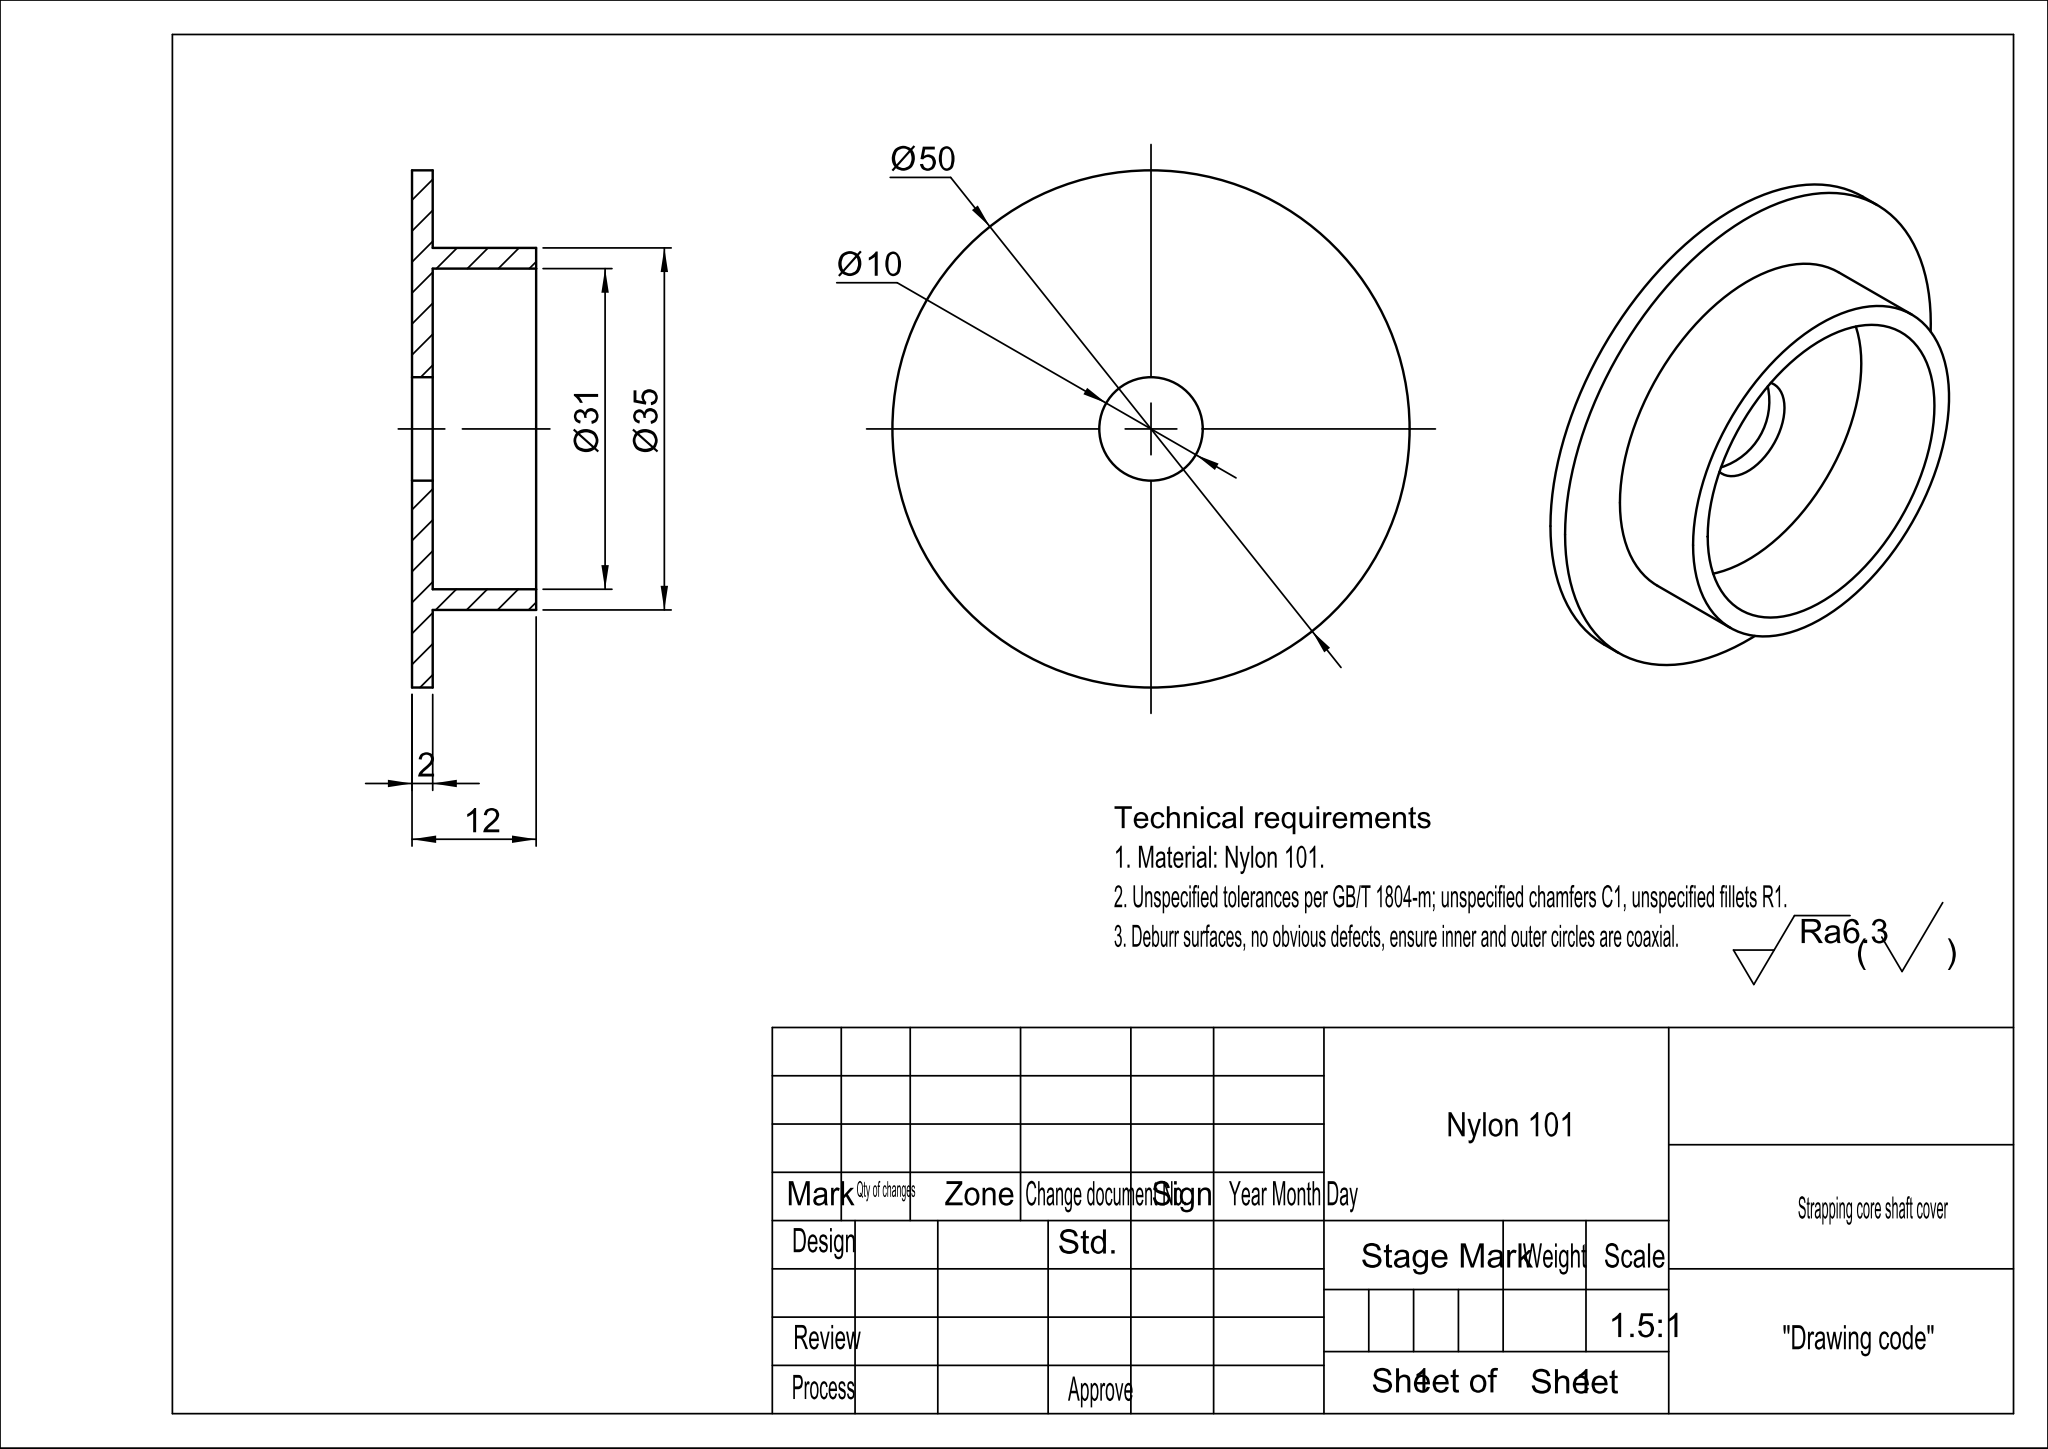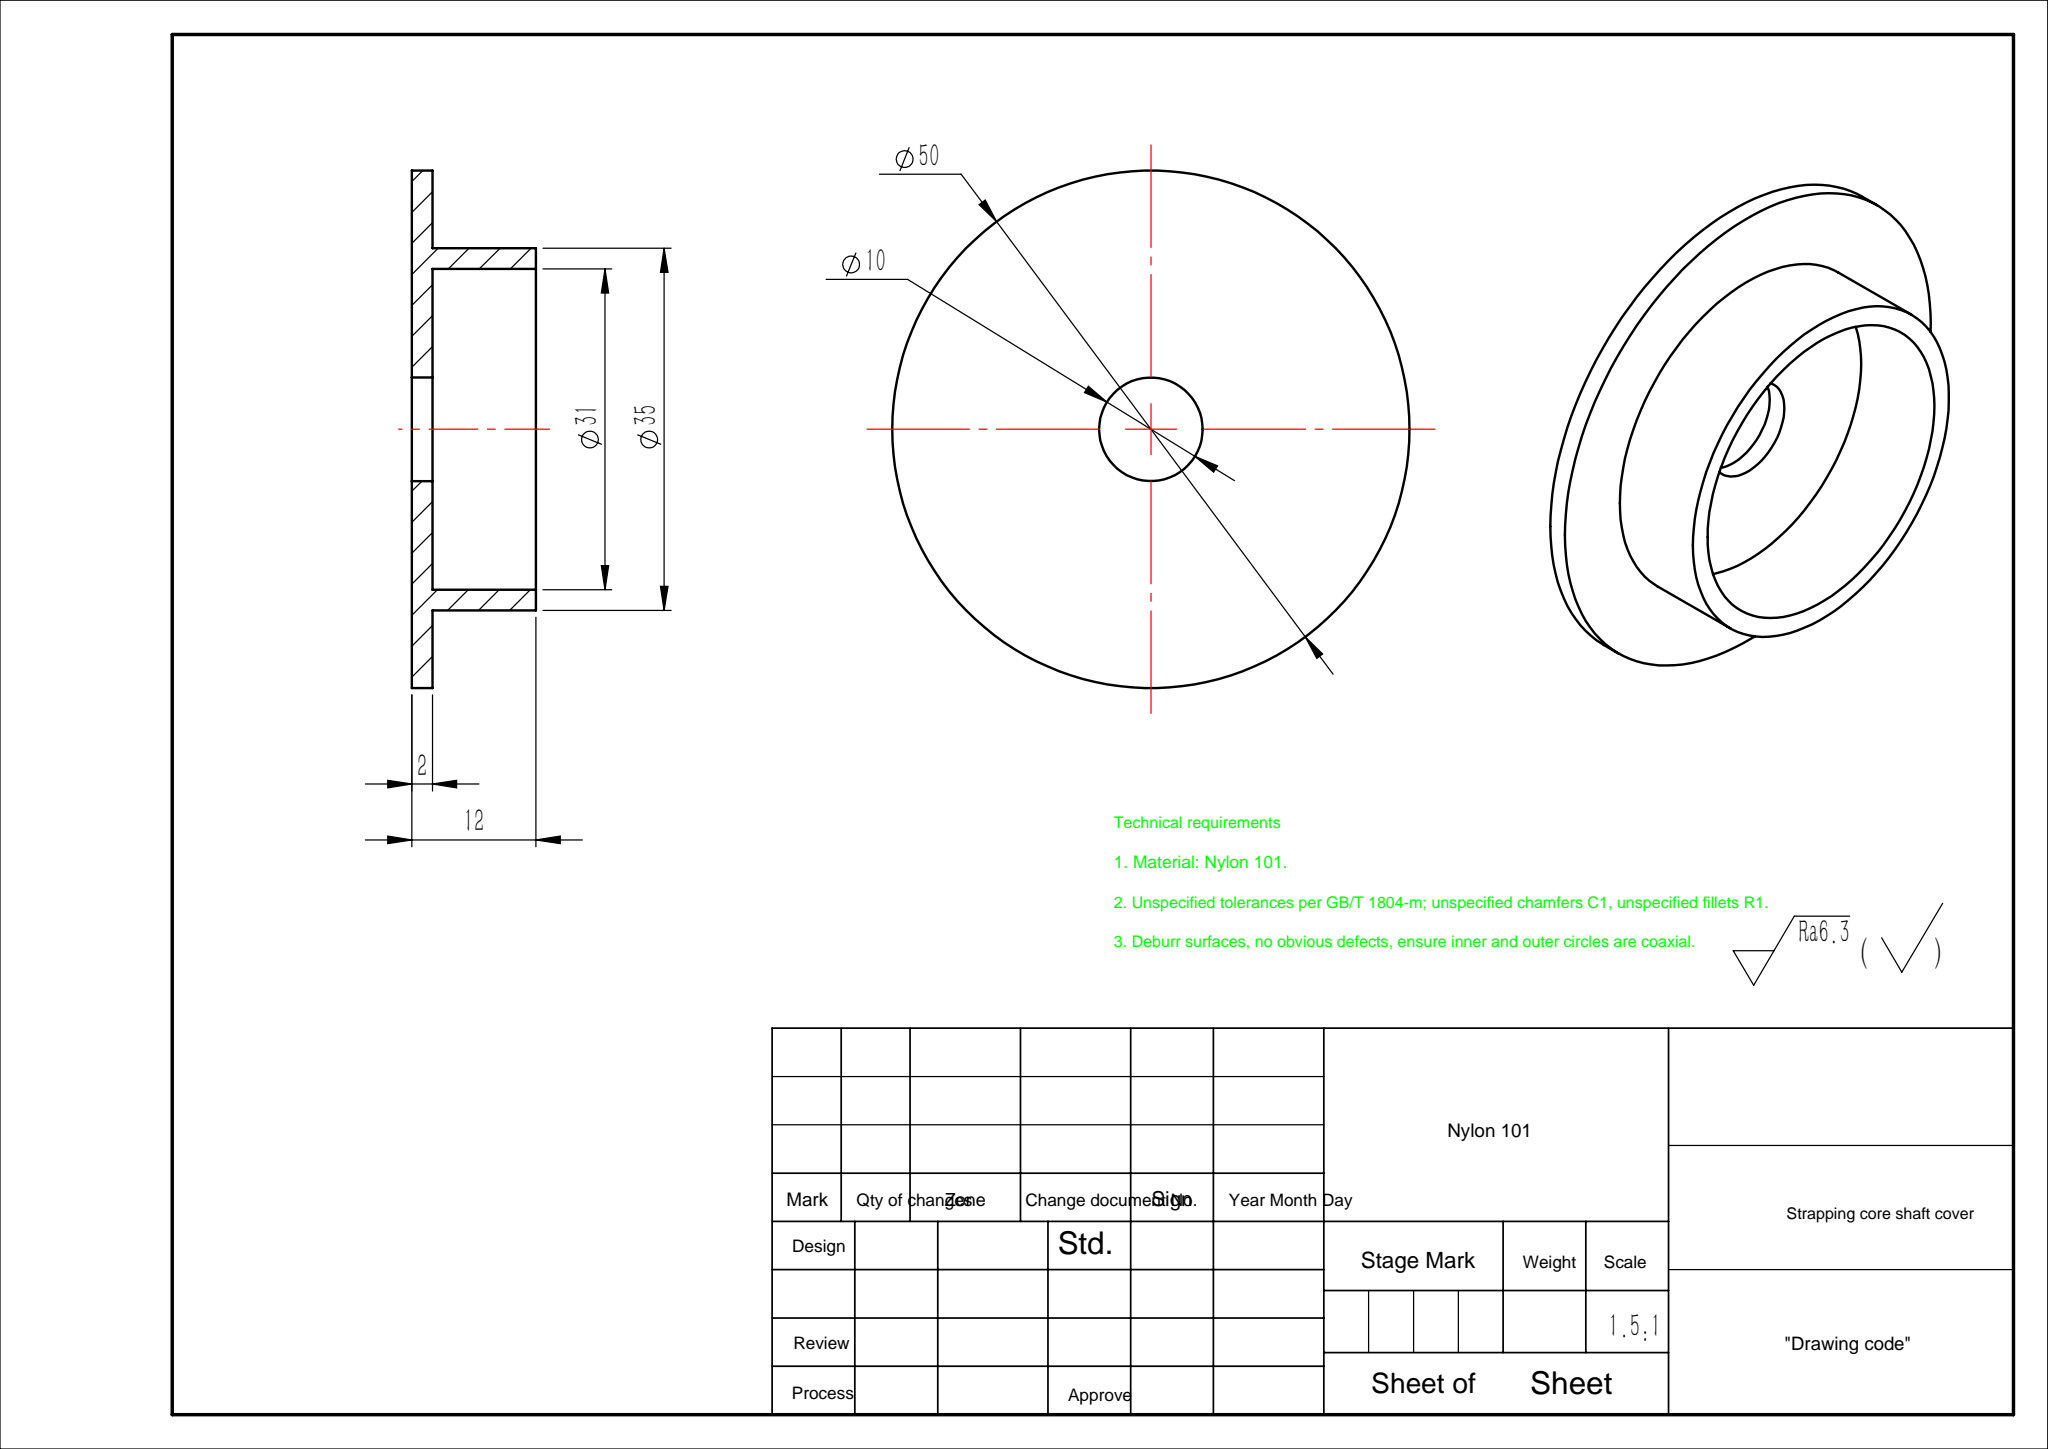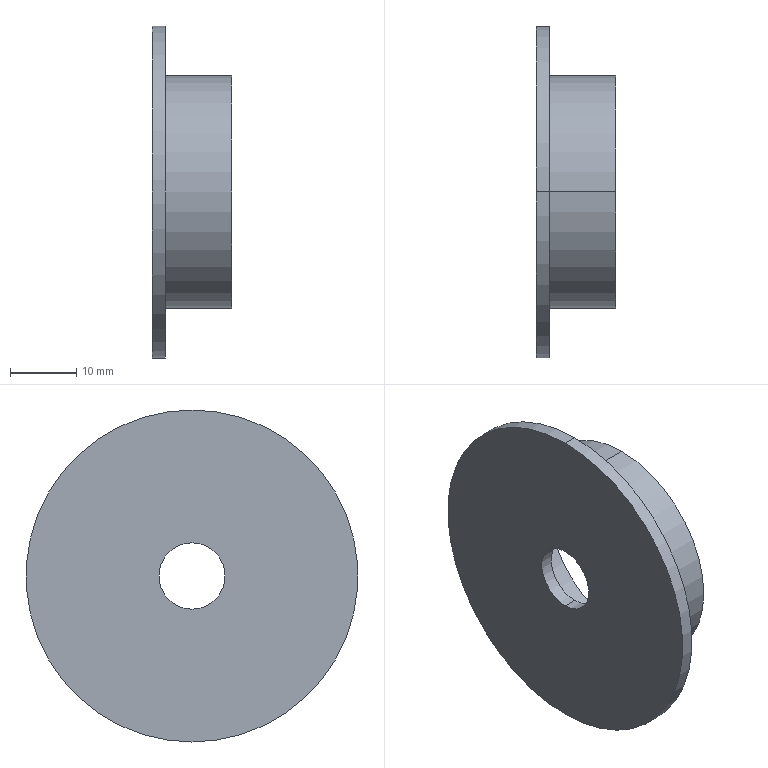Part | SolidWorks | features Revolution 1 | 1 solid | 12 faces | box 12 x 50 x 50 mm | volume 5843 mm3 | cylinder 8 | plane 4 | commonest cylinder face diameters 10 x2 31 x2 35 x2 50 x2
STEP:
#1=CARTESIAN_POINT('',(2.,0.,-5.));
#2=VERTEX_POINT('',#1);
#3=CARTESIAN_POINT('',(2.,0.,5.));
#4=VERTEX_POINT('',#3);
#5=CARTESIAN_POINT('',(2.,0.,0.));
#6=DIRECTION('',(-1.,0.,0.));
#7=DIRECTION('',(0.,0.,1.));
#8=AXIS2_PLACEMENT_3D('',#5,#6,#7);
#9=CIRCLE('',#8,5.);
#10=EDGE_CURVE('',#2,#4,#9,.T.);
#11=ORIENTED_EDGE('',*,*,#10,.F.);
#12=CARTESIAN_POINT('',(0.,0.,-5.));
#13=VERTEX_POINT('',#12);
#14=CARTESIAN_POINT('',(0.,0.,-5.));
#15=DIRECTION('',(-1.,0.,0.));
#16=VECTOR('',#15,1000.);
#17=LINE('',#14,#16);
#18=EDGE_CURVE('',#2,#13,#17,.T.);
#19=ORIENTED_EDGE('',*,*,#18,.T.);
#20=CARTESIAN_POINT('',(0.,0.,5.));
#21=VERTEX_POINT('',#20);
#22=CARTESIAN_POINT('',(0.,0.,0.));
#23=DIRECTION('',(-1.,0.,0.));
#24=DIRECTION('',(0.,0.,1.));
#25=AXIS2_PLACEMENT_3D('',#22,#23,#24);
#26=CIRCLE('',#25,5.);
#27=EDGE_CURVE('',#13,#21,#26,.T.);
#28=ORIENTED_EDGE('',*,*,#27,.T.);
#29=CARTESIAN_POINT('',(0.,0.,5.));
#30=DIRECTION('',(-1.,0.,0.));
#31=VECTOR('',#30,1000.);
#32=LINE('',#29,#31);
#33=EDGE_CURVE('',#4,#21,#32,.T.);
#34=ORIENTED_EDGE('',*,*,#33,.F.);
#35=EDGE_LOOP('',(#11,#19,#28,#34));
#36=FACE_OUTER_BOUND('',#35,.T.);
#37=CARTESIAN_POINT('',(0.,0.,0.));
#38=DIRECTION('',(-1.,0.,0.));
#39=DIRECTION('',(0.,0.,1.));
#40=AXIS2_PLACEMENT_3D('',#37,#38,#39);
#41=CYLINDRICAL_SURFACE('',#40,5.);
#42=ADVANCED_FACE('',(#36),#41,.F.);
#43=CARTESIAN_POINT('',(12.,0.,-15.5));
#44=VERTEX_POINT('',#43);
#45=CARTESIAN_POINT('',(12.,0.,15.5));
#46=VERTEX_POINT('',#45);
#47=CARTESIAN_POINT('',(12.,0.,0.));
#48=DIRECTION('',(-1.,0.,0.));
#49=DIRECTION('',(0.,0.,1.));
#50=AXIS2_PLACEMENT_3D('',#47,#48,#49);
#51=CIRCLE('',#50,15.5);
#52=EDGE_CURVE('',#44,#46,#51,.T.);
#53=ORIENTED_EDGE('',*,*,#52,.F.);
#54=CARTESIAN_POINT('',(2.,0.,-15.5));
#55=VERTEX_POINT('',#54);
#56=CARTESIAN_POINT('',(0.,0.,-15.5));
#57=DIRECTION('',(-1.,0.,0.));
#58=VECTOR('',#57,1000.);
#59=LINE('',#56,#58);
#60=EDGE_CURVE('',#44,#55,#59,.T.);
#61=ORIENTED_EDGE('',*,*,#60,.T.);
#62=CARTESIAN_POINT('',(2.,0.,15.5));
#63=VERTEX_POINT('',#62);
#64=CARTESIAN_POINT('',(2.,0.,0.));
#65=DIRECTION('',(-1.,0.,0.));
#66=DIRECTION('',(0.,0.,1.));
#67=AXIS2_PLACEMENT_3D('',#64,#65,#66);
#68=CIRCLE('',#67,15.5);
#69=EDGE_CURVE('',#55,#63,#68,.T.);
#70=ORIENTED_EDGE('',*,*,#69,.T.);
#71=CARTESIAN_POINT('',(0.,0.,15.5));
#72=DIRECTION('',(-1.,0.,0.));
#73=VECTOR('',#72,1000.);
#74=LINE('',#71,#73);
#75=EDGE_CURVE('',#46,#63,#74,.T.);
#76=ORIENTED_EDGE('',*,*,#75,.F.);
#77=EDGE_LOOP('',(#53,#61,#70,#76));
#78=FACE_OUTER_BOUND('',#77,.T.);
#79=CARTESIAN_POINT('',(0.,0.,0.));
#80=DIRECTION('',(-1.,0.,0.));
#81=DIRECTION('',(0.,0.,1.));
#82=AXIS2_PLACEMENT_3D('',#79,#80,#81);
#83=CYLINDRICAL_SURFACE('',#82,15.5);
#84=ADVANCED_FACE('',(#78),#83,.F.);
#85=CARTESIAN_POINT('',(12.,0.,17.5));
#86=VERTEX_POINT('',#85);
#87=CARTESIAN_POINT('',(12.,0.,-17.5));
#88=VERTEX_POINT('',#87);
#89=CARTESIAN_POINT('',(12.,0.,0.));
#90=DIRECTION('',(-1.,0.,0.));
#91=DIRECTION('',(0.,0.,1.));
#92=AXIS2_PLACEMENT_3D('',#89,#90,#91);
#93=CIRCLE('',#92,17.5);
#94=EDGE_CURVE('',#86,#88,#93,.T.);
#95=ORIENTED_EDGE('',*,*,#94,.T.);
#96=CARTESIAN_POINT('',(2.,0.,-17.5));
#97=VERTEX_POINT('',#96);
#98=CARTESIAN_POINT('',(0.,0.,-17.5));
#99=DIRECTION('',(-1.,0.,0.));
#100=VECTOR('',#99,1000.);
#101=LINE('',#98,#100);
#102=EDGE_CURVE('',#88,#97,#101,.T.);
#103=ORIENTED_EDGE('',*,*,#102,.T.);
#104=CARTESIAN_POINT('',(2.,0.,17.5));
#105=VERTEX_POINT('',#104);
#106=CARTESIAN_POINT('',(2.,0.,0.));
#107=DIRECTION('',(-1.,0.,0.));
#108=DIRECTION('',(0.,0.,1.));
#109=AXIS2_PLACEMENT_3D('',#106,#107,#108);
#110=CIRCLE('',#109,17.5);
#111=EDGE_CURVE('',#105,#97,#110,.T.);
#112=ORIENTED_EDGE('',*,*,#111,.F.);
#113=CARTESIAN_POINT('',(0.,0.,17.5));
#114=DIRECTION('',(-1.,0.,0.));
#115=VECTOR('',#114,1000.);
#116=LINE('',#113,#115);
#117=EDGE_CURVE('',#86,#105,#116,.T.);
#118=ORIENTED_EDGE('',*,*,#117,.F.);
#119=EDGE_LOOP('',(#95,#103,#112,#118));
#120=FACE_OUTER_BOUND('',#119,.T.);
#121=CARTESIAN_POINT('',(0.,0.,0.));
#122=DIRECTION('',(-1.,0.,0.));
#123=DIRECTION('',(0.,0.,1.));
#124=AXIS2_PLACEMENT_3D('',#121,#122,#123);
#125=CYLINDRICAL_SURFACE('',#124,17.5);
#126=ADVANCED_FACE('',(#120),#125,.T.);
#127=CARTESIAN_POINT('',(2.,0.,25.));
#128=VERTEX_POINT('',#127);
#129=CARTESIAN_POINT('',(2.,0.,-25.));
#130=VERTEX_POINT('',#129);
#131=CARTESIAN_POINT('',(2.,0.,0.));
#132=DIRECTION('',(-1.,0.,0.));
#133=DIRECTION('',(0.,0.,1.));
#134=AXIS2_PLACEMENT_3D('',#131,#132,#133);
#135=CIRCLE('',#134,25.);
#136=EDGE_CURVE('',#128,#130,#135,.T.);
#137=ORIENTED_EDGE('',*,*,#136,.T.);
#138=CARTESIAN_POINT('',(0.,0.,-25.));
#139=VERTEX_POINT('',#138);
#140=CARTESIAN_POINT('',(0.,0.,-25.));
#141=DIRECTION('',(-1.,0.,0.));
#142=VECTOR('',#141,1000.);
#143=LINE('',#140,#142);
#144=EDGE_CURVE('',#130,#139,#143,.T.);
#145=ORIENTED_EDGE('',*,*,#144,.T.);
#146=CARTESIAN_POINT('',(0.,0.,25.));
#147=VERTEX_POINT('',#146);
#148=CARTESIAN_POINT('',(0.,0.,0.));
#149=DIRECTION('',(-1.,0.,0.));
#150=DIRECTION('',(0.,0.,1.));
#151=AXIS2_PLACEMENT_3D('',#148,#149,#150);
#152=CIRCLE('',#151,25.);
#153=EDGE_CURVE('',#147,#139,#152,.T.);
#154=ORIENTED_EDGE('',*,*,#153,.F.);
#155=CARTESIAN_POINT('',(0.,0.,25.));
#156=DIRECTION('',(-1.,0.,0.));
#157=VECTOR('',#156,1000.);
#158=LINE('',#155,#157);
#159=EDGE_CURVE('',#128,#147,#158,.T.);
#160=ORIENTED_EDGE('',*,*,#159,.F.);
#161=EDGE_LOOP('',(#137,#145,#154,#160));
#162=FACE_OUTER_BOUND('',#161,.T.);
#163=CARTESIAN_POINT('',(0.,0.,0.));
#164=DIRECTION('',(-1.,0.,0.));
#165=DIRECTION('',(0.,0.,1.));
#166=AXIS2_PLACEMENT_3D('',#163,#164,#165);
#167=CYLINDRICAL_SURFACE('',#166,25.);
#168=ADVANCED_FACE('',(#162),#167,.T.);
#169=CARTESIAN_POINT('',(0.,0.,0.));
#170=DIRECTION('',(-1.,0.,0.));
#171=DIRECTION('',(0.,0.,1.));
#172=AXIS2_PLACEMENT_3D('',#169,#170,#171);
#173=CIRCLE('',#172,5.);
#174=EDGE_CURVE('',#21,#13,#173,.T.);
#175=ORIENTED_EDGE('',*,*,#174,.F.);
#176=ORIENTED_EDGE('',*,*,#27,.F.);
#177=EDGE_LOOP('',(#175,#176));
#178=FACE_BOUND('',#177,.T.);
#179=ORIENTED_EDGE('',*,*,#153,.T.);
#180=CARTESIAN_POINT('',(0.,0.,0.));
#181=DIRECTION('',(-1.,0.,0.));
#182=DIRECTION('',(0.,0.,1.));
#183=AXIS2_PLACEMENT_3D('',#180,#181,#182);
#184=CIRCLE('',#183,25.);
#185=EDGE_CURVE('',#139,#147,#184,.T.);
#186=ORIENTED_EDGE('',*,*,#185,.T.);
#187=EDGE_LOOP('',(#179,#186));
#188=FACE_OUTER_BOUND('',#187,.T.);
#189=CARTESIAN_POINT('',(0.,5.,0.));
#190=DIRECTION('',(1.,0.,0.));
#191=DIRECTION('',(0.,0.,-1.));
#192=AXIS2_PLACEMENT_3D('',#189,#190,#191);
#193=PLANE('',#192);
#194=ADVANCED_FACE('',(#178,#188),#193,.F.);
#195=ORIENTED_EDGE('',*,*,#144,.F.);
#196=CARTESIAN_POINT('',(2.,0.,0.));
#197=DIRECTION('',(-1.,0.,0.));
#198=DIRECTION('',(0.,0.,1.));
#199=AXIS2_PLACEMENT_3D('',#196,#197,#198);
#200=CIRCLE('',#199,25.);
#201=EDGE_CURVE('',#130,#128,#200,.T.);
#202=ORIENTED_EDGE('',*,*,#201,.T.);
#203=ORIENTED_EDGE('',*,*,#159,.T.);
#204=ORIENTED_EDGE('',*,*,#185,.F.);
#205=EDGE_LOOP('',(#195,#202,#203,#204));
#206=FACE_OUTER_BOUND('',#205,.T.);
#207=CARTESIAN_POINT('',(0.,0.,0.));
#208=DIRECTION('',(-1.,0.,0.));
#209=DIRECTION('',(0.,0.,1.));
#210=AXIS2_PLACEMENT_3D('',#207,#208,#209);
#211=CYLINDRICAL_SURFACE('',#210,25.);
#212=ADVANCED_FACE('',(#206),#211,.T.);
#213=ORIENTED_EDGE('',*,*,#136,.F.);
#214=ORIENTED_EDGE('',*,*,#201,.F.);
#215=EDGE_LOOP('',(#213,#214));
#216=FACE_OUTER_BOUND('',#215,.T.);
#217=ORIENTED_EDGE('',*,*,#111,.T.);
#218=CARTESIAN_POINT('',(2.,0.,0.));
#219=DIRECTION('',(-1.,0.,0.));
#220=DIRECTION('',(0.,0.,1.));
#221=AXIS2_PLACEMENT_3D('',#218,#219,#220);
#222=CIRCLE('',#221,17.5);
#223=EDGE_CURVE('',#97,#105,#222,.T.);
#224=ORIENTED_EDGE('',*,*,#223,.T.);
#225=EDGE_LOOP('',(#217,#224));
#226=FACE_BOUND('',#225,.T.);
#227=CARTESIAN_POINT('',(2.,25.,0.));
#228=DIRECTION('',(-1.,0.,0.));
#229=DIRECTION('',(0.,0.,1.));
#230=AXIS2_PLACEMENT_3D('',#227,#228,#229);
#231=PLANE('',#230);
#232=ADVANCED_FACE('',(#216,#226),#231,.F.);
#233=ORIENTED_EDGE('',*,*,#102,.F.);
#234=CARTESIAN_POINT('',(12.,0.,0.));
#235=DIRECTION('',(-1.,0.,0.));
#236=DIRECTION('',(0.,0.,1.));
#237=AXIS2_PLACEMENT_3D('',#234,#235,#236);
#238=CIRCLE('',#237,17.5);
#239=EDGE_CURVE('',#88,#86,#238,.T.);
#240=ORIENTED_EDGE('',*,*,#239,.T.);
#241=ORIENTED_EDGE('',*,*,#117,.T.);
#242=ORIENTED_EDGE('',*,*,#223,.F.);
#243=EDGE_LOOP('',(#233,#240,#241,#242));
#244=FACE_OUTER_BOUND('',#243,.T.);
#245=CARTESIAN_POINT('',(0.,0.,0.));
#246=DIRECTION('',(-1.,0.,0.));
#247=DIRECTION('',(0.,0.,1.));
#248=AXIS2_PLACEMENT_3D('',#245,#246,#247);
#249=CYLINDRICAL_SURFACE('',#248,17.5);
#250=ADVANCED_FACE('',(#244),#249,.T.);
#251=ORIENTED_EDGE('',*,*,#94,.F.);
#252=ORIENTED_EDGE('',*,*,#239,.F.);
#253=EDGE_LOOP('',(#251,#252));
#254=FACE_OUTER_BOUND('',#253,.T.);
#255=CARTESIAN_POINT('',(12.,0.,0.));
#256=DIRECTION('',(-1.,0.,0.));
#257=DIRECTION('',(0.,0.,1.));
#258=AXIS2_PLACEMENT_3D('',#255,#256,#257);
#259=CIRCLE('',#258,15.5);
#260=EDGE_CURVE('',#46,#44,#259,.T.);
#261=ORIENTED_EDGE('',*,*,#260,.T.);
#262=ORIENTED_EDGE('',*,*,#52,.T.);
#263=EDGE_LOOP('',(#261,#262));
#264=FACE_BOUND('',#263,.T.);
#265=CARTESIAN_POINT('',(12.,17.5,0.));
#266=DIRECTION('',(-1.,0.,0.));
#267=DIRECTION('',(0.,0.,1.));
#268=AXIS2_PLACEMENT_3D('',#265,#266,#267);
#269=PLANE('',#268);
#270=ADVANCED_FACE('',(#254,#264),#269,.F.);
#271=ORIENTED_EDGE('',*,*,#60,.F.);
#272=ORIENTED_EDGE('',*,*,#260,.F.);
#273=ORIENTED_EDGE('',*,*,#75,.T.);
#274=CARTESIAN_POINT('',(2.,0.,0.));
#275=DIRECTION('',(-1.,0.,0.));
#276=DIRECTION('',(0.,0.,1.));
#277=AXIS2_PLACEMENT_3D('',#274,#275,#276);
#278=CIRCLE('',#277,15.5);
#279=EDGE_CURVE('',#63,#55,#278,.T.);
#280=ORIENTED_EDGE('',*,*,#279,.T.);
#281=EDGE_LOOP('',(#271,#272,#273,#280));
#282=FACE_OUTER_BOUND('',#281,.T.);
#283=CARTESIAN_POINT('',(0.,0.,0.));
#284=DIRECTION('',(-1.,0.,0.));
#285=DIRECTION('',(0.,0.,1.));
#286=AXIS2_PLACEMENT_3D('',#283,#284,#285);
#287=CYLINDRICAL_SURFACE('',#286,15.5);
#288=ADVANCED_FACE('',(#282),#287,.F.);
#289=ORIENTED_EDGE('',*,*,#279,.F.);
#290=ORIENTED_EDGE('',*,*,#69,.F.);
#291=EDGE_LOOP('',(#289,#290));
#292=FACE_OUTER_BOUND('',#291,.T.);
#293=CARTESIAN_POINT('',(2.,0.,0.));
#294=DIRECTION('',(-1.,0.,0.));
#295=DIRECTION('',(0.,0.,1.));
#296=AXIS2_PLACEMENT_3D('',#293,#294,#295);
#297=CIRCLE('',#296,5.);
#298=EDGE_CURVE('',#4,#2,#297,.T.);
#299=ORIENTED_EDGE('',*,*,#298,.T.);
#300=ORIENTED_EDGE('',*,*,#10,.T.);
#301=EDGE_LOOP('',(#299,#300));
#302=FACE_BOUND('',#301,.T.);
#303=CARTESIAN_POINT('',(2.,15.5,0.));
#304=DIRECTION('',(-1.,0.,0.));
#305=DIRECTION('',(0.,0.,1.));
#306=AXIS2_PLACEMENT_3D('',#303,#304,#305);
#307=PLANE('',#306);
#308=ADVANCED_FACE('',(#292,#302),#307,.F.);
#309=ORIENTED_EDGE('',*,*,#18,.F.);
#310=ORIENTED_EDGE('',*,*,#298,.F.);
#311=ORIENTED_EDGE('',*,*,#33,.T.);
#312=ORIENTED_EDGE('',*,*,#174,.T.);
#313=EDGE_LOOP('',(#309,#310,#311,#312));
#314=FACE_OUTER_BOUND('',#313,.T.);
#315=CARTESIAN_POINT('',(0.,0.,0.));
#316=DIRECTION('',(-1.,0.,0.));
#317=DIRECTION('',(0.,0.,1.));
#318=AXIS2_PLACEMENT_3D('',#315,#316,#317);
#319=CYLINDRICAL_SURFACE('',#318,5.);
#320=ADVANCED_FACE('',(#314),#319,.F.);
#321=CLOSED_SHELL('',(#42,#84,#126,#168,#194,#212,#232,#250,#270,#288,#308,#320));
#322=MANIFOLD_SOLID_BREP('',#321);
#323=CARTESIAN_POINT('',(0.,0.,0.));
#324=DIRECTION('',(0.,0.,1.));
#325=DIRECTION('',(1.,0.,0.));
#326=AXIS2_PLACEMENT_3D('',#323,#324,#325);
#327=(LENGTH_UNIT()NAMED_UNIT(*)SI_UNIT(.MILLI.,.METRE.));
#328=UNCERTAINTY_MEASURE_WITH_UNIT(LENGTH_MEASURE(0.00001),#327,'','');
#329=(NAMED_UNIT(*)PLANE_ANGLE_UNIT()SI_UNIT($,.RADIAN.));
#330=(NAMED_UNIT(*)SI_UNIT($,.STERADIAN.)SOLID_ANGLE_UNIT());
#331=(GEOMETRIC_REPRESENTATION_CONTEXT(3)GLOBAL_UNCERTAINTY_ASSIGNED_CONTEXT((#328))GLOBAL_UNIT_ASSIGNED_CONTEXT((#327,#329,#330))REPRESENTATION_CONTEXT('',''));
#332=ADVANCED_BREP_SHAPE_REPRESENTATION('',(#322,#326),#331);